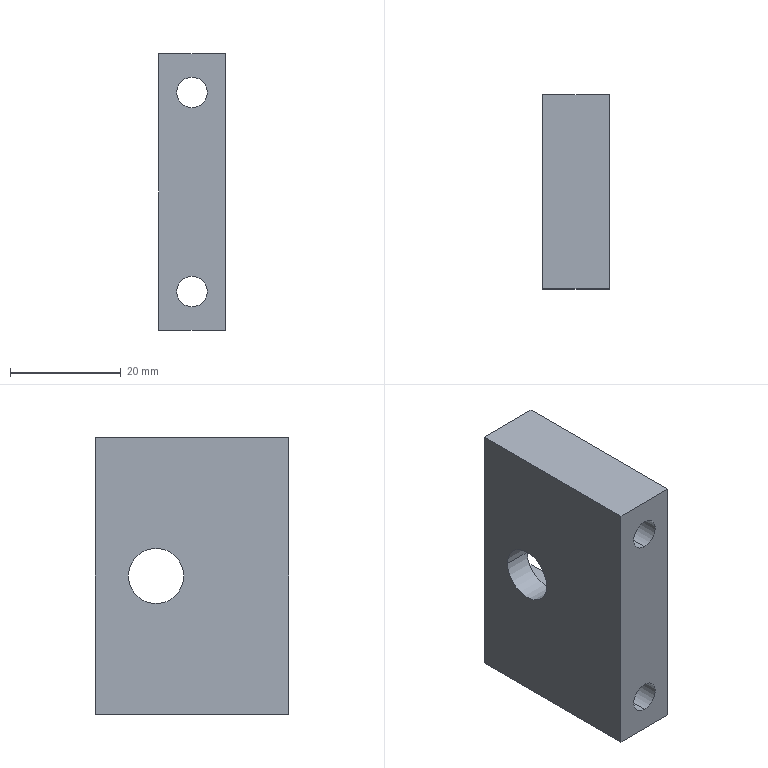Part | STEP file | slideway cylinder seat | 1 solid | 24 faces | box 12 x 35 x 50 mm | volume 15461 mm3 | cylinder 12 | plane 12 | commonest cylinder face diameters 10 x6 5.5 x4 12 x2